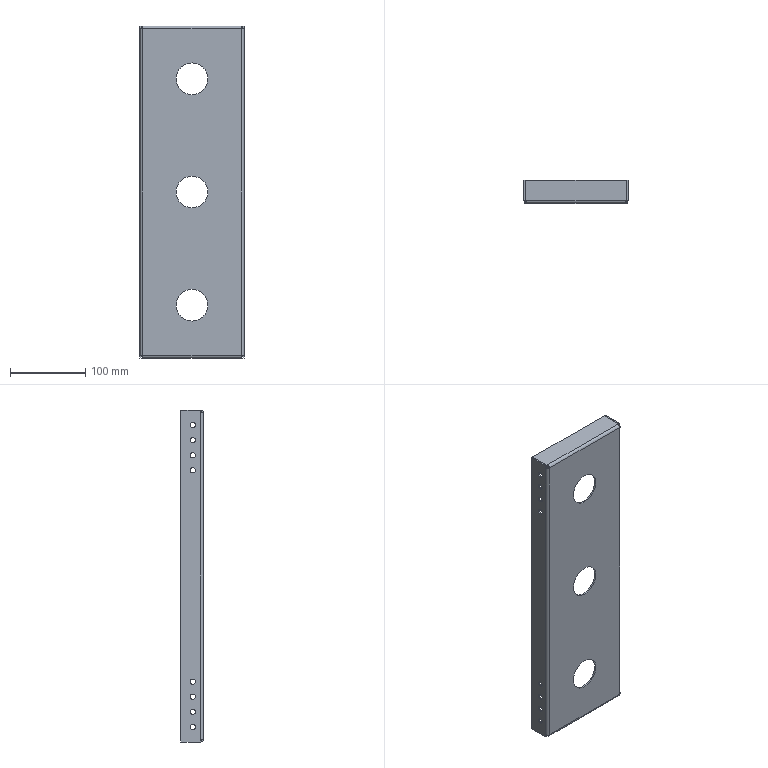Part | STEP file | 1 solid | 84 faces | box 138 x 30 x 440 mm | volume 173584 mm3 | cylinder 46 | plane 38 | commonest cylinder face diameters 7 x36 42 x6 3 x4